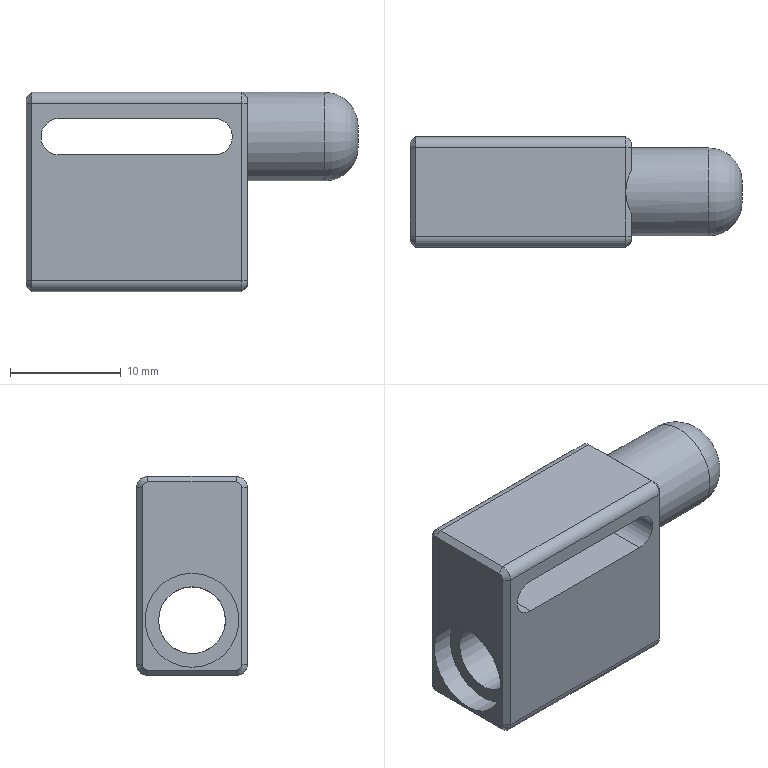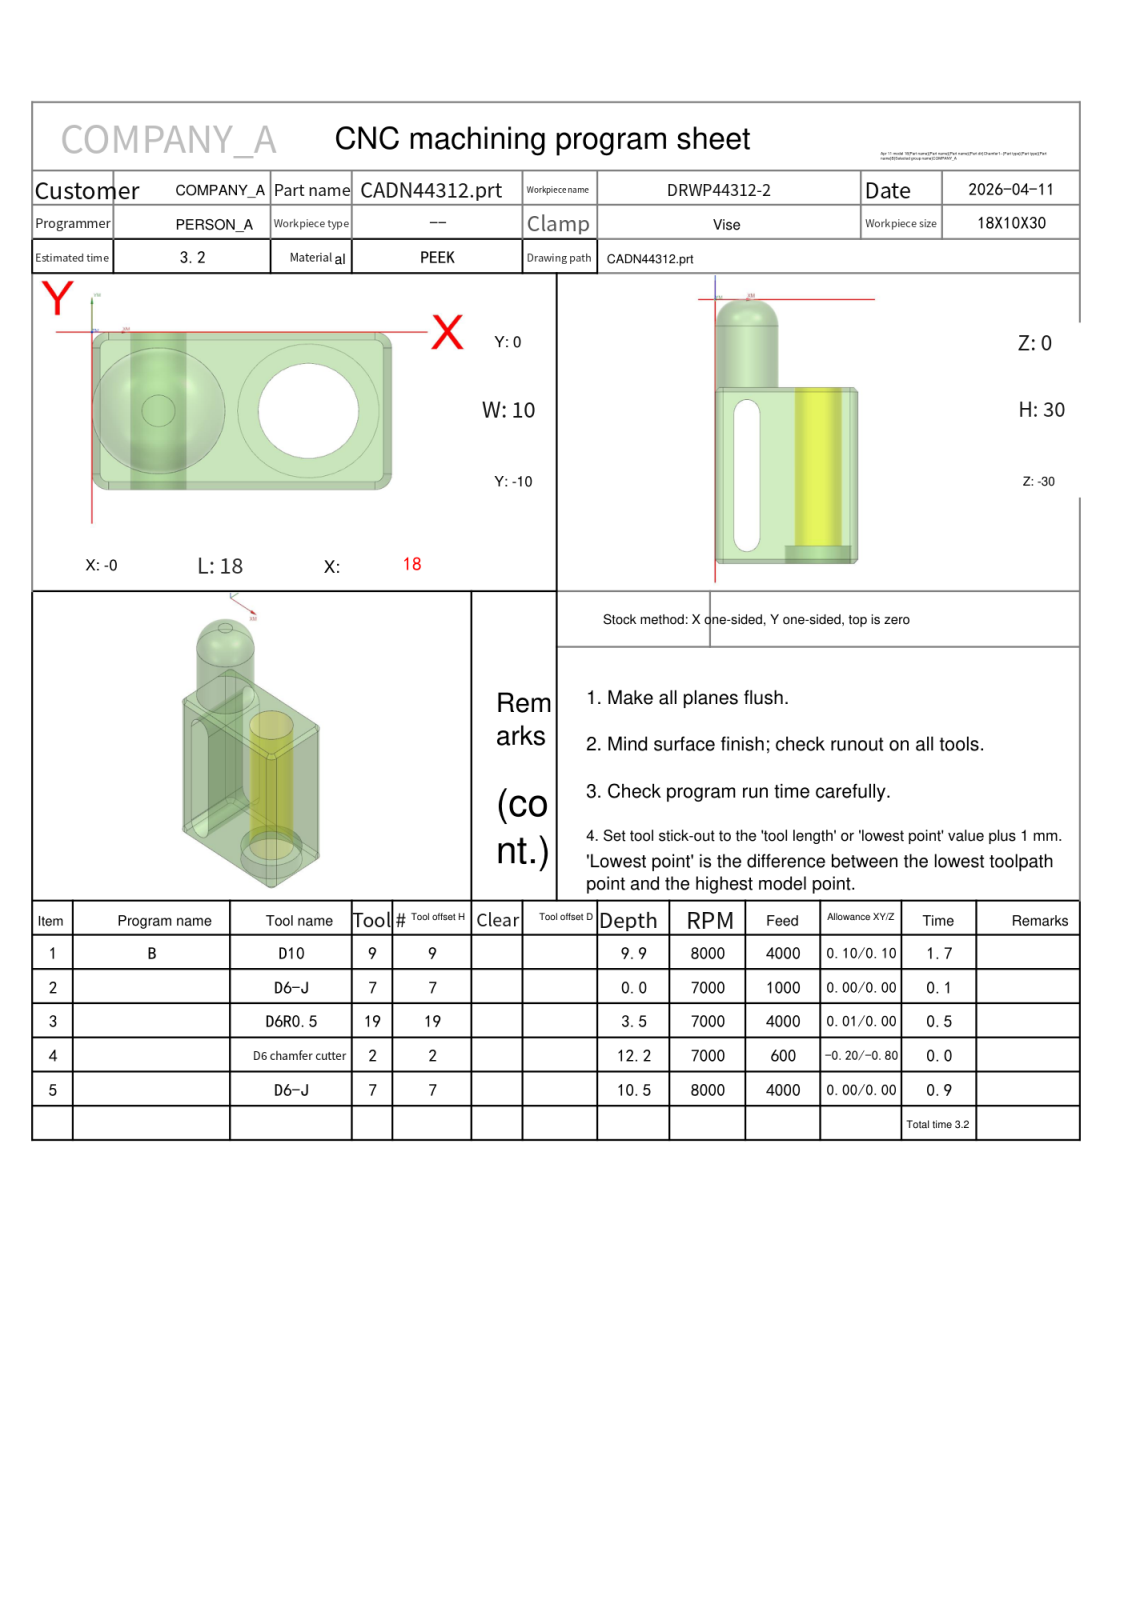NC program | NX | posted by the shop | part box 30 x 10 x 18 mm
Lines 1 to 1408 of 11854:
%
O0001
(Machine time: 4.17 MIN)
(===Total Tool:4===)
(T9=D10     D=10.  R=0.   D-  H09 Z=-9.9  )
(T7=D6-J    D=6.   R=0.   D-  H07 Z=-10.5 )
(T19=D6R0.5 D=6.   R=0.5  D-  H19 Z=-3.5  )
(T2=D6 chamfer cutter    D=6.   R=0.   D-  H02 Z=-12.2 )
G80 G90 G17 G49 G40
G91 G28 Z0
M01
N1 T09 M06
(D10  D=10. R=0. H=09 ce=0.20 di=0.10)
G00 G90 G54 X-17. Y-1.667 M03 S8000
G43 H09 Z20.
M08
Z6.011
G01 Z4.011 F3000.
X-5.
X22.
G02 X23. Y-2.666 I0.0 J-1.
G01 Y-7.433
G02 X22.1 Y-8.333 I-.9 J0.0
G01 X-5.
X-17.
Z6.011
G00 Z7.5
Y-1.667
Z5.522
G01 Z3.522
X-5.
X22.
G02 X23. Y-2.666 I0.0 J-1.
G01 Y-7.433
G02 X22.1 Y-8.333 I-.9 J0.0
G01 X-5.
X-17.
Z5.522
G00 Z7.011
Y-1.667
Z5.033
G01 Z3.033
X-5.
X22.
G02 X23. Y-2.666 I0.0 J-1.
G01 Y-7.433
G02 X22.1 Y-8.333 I-.9 J0.0
G01 X-5.
X-17.
Z5.033
G00 Z6.522
Y-1.667
Z4.544
G01 Z2.544
X-5.
X22.
G02 X23. Y-2.666 I0.0 J-1.
G01 Y-7.433
G02 X22.1 Y-8.333 I-.9 J0.0
G01 X-5.
X-17.
Z4.544
G00 Z6.033
Y-1.667
Z4.056
G01 Z2.056
X-5.
X22.
G02 X23. Y-2.666 I0.0 J-1.
G01 Y-7.433
G02 X22.1 Y-8.333 I-.9 J0.0
G01 X-5.
X-17.
Z4.056
G00 Z5.544
Y-1.667
Z3.567
G01 Z1.567
X-5.
X22.
G02 X23. Y-2.666 I0.0 J-1.
G01 Y-7.433
G02 X22.1 Y-8.333 I-.9 J0.0
G01 X-5.
X-17.
Z3.567
G00 Z5.056
Y-1.667
Z3.078
G01 Z1.078
X-5.
X22.
G02 X23. Y-2.666 I0.0 J-1.
G01 Y-7.433
G02 X22.1 Y-8.333 I-.9 J0.0
G01 X-5.
X-17.
Z3.078
G00 Z4.567
Y-1.667
Z2.589
G01 Z.589
X-5.
X22.
G02 X23. Y-2.666 I0.0 J-1.
G01 Y-7.433
G02 X22.1 Y-8.333 I-.9 J0.0
G01 X-5.
X-17.
Z2.589
G00 Z4.078
Y-1.667
Z2.1
G01 Z.1
X-5.
X22.
G02 X23. Y-2.666 I0.0 J-1.
G01 Y-7.433
G02 X22.1 Y-8.333 I-.9 J0.0
G01 X-5.
X-17.
Z2.1
G00 Z20.
G00 G90 X7.765 Y13. M03 S8000
Z14.8
Z.804
G01 Z-.396 F4000.
Y8.5
G03 X14.765 Y1.5 I7. J0.0
G01 X19.429
X20.55 Y1.496
G02 X20.998 Y1.048 I-.048 J-.495
G01 Y-11.048
G02 X20.55 Y-11.496 I-.495 J.047
G01 X19.43 Y-11.499
X10.345 Y-11.498
G02 X4. Y-14.082 I-6.345 J6.498
X-2.347 Y-11.496 I0.0 J9.082
G01 X-2.553
G02 X-2.998 Y-11.048 I.051 J.495
G01 Y-10.789
G02 X-5.082 Y-5. I6.998 J5.789
X-2.998 Y.789 I9.082 J0.0
G01 Y1.048
G02 X-2.55 Y1.496 I.495 J-.047
G01 X-2.346 Y1.497
G02 X4. Y4.082 I6.346 J-6.497
X10.343 Y1.5 I0.0 J-9.082
G01 X14.031
G02 X14.99 Y.785 I0.0 J-1.
G01 X16.144 Y-3.092
G03 X16.3 Y-3.403 I.958 J.286
G02 X16.498 Y-3.999 I-.802 J-.597
G01 Y-6.
G02 X15.499 Y-6.999 I-1. J.001
G01 X14.031
G02 X13.032 Y-5.999 I.001 J1.
G01 X13.037 Y-5.901
G03 X13.082 Y-5. I-9.037 J.901
X13.079 Y-4.775 I-9.082 J0.0
X12.449 Y-4.16 I-.63 J-.016
G01 X12.387 Y-4.163
X12.354 Y-4.167
G03 X11.682 Y-4.91 I.074 J-.743
G01 Y-4.917
Y-5.
G02 X4. Y-12.682 I-7.682 J0.0
X-3.682 Y-5. I0.0 J7.682
X4. Y2.682 I7.682 J0.0
X11.644 Y-4.238 I0.0 J-7.682
G03 X12.062 Y-4.616 I.418 J.042
X12.279 Y-4.556 I0.0 J.42
G01 X12.846 Y-4.214
G03 X13.036 Y-3.91 I-.205 J.34
G02 X14.031 Y-3. I.996 J-.091
G01 X14.531
G03 X21.531 Y3.999 I0.0 J7.
G01 Y12.955
Z.804
G00 Z3.
G01 X32.458 Y2. F6000.
G00 Z.408
G01 Z-.792 F4000.
X27.998
G03 X20.998 Y-5. I0.0 J-7.
G01 Y-11.048
G02 X20.55 Y-11.496 I-.496 J.047
G01 X19.43 Y-11.5
X11.034 Y-11.498
G02 X4. Y-14.576 I-7.034 J6.498
X-5.576 Y-5. I0.0 J9.576
X4. Y4.576 I9.576 J0.0
X11.032 Y1.5 I0.0 J-9.576
G01 X19.43
X20.55 Y1.496
G02 X20.998 Y1.048 I-.048 J-.495
G01 Y-10.
G02 X19.998 Y-11. I-1. J0.0
X19.383 Y-10.788 I0.0 J1.
G01 X15.112 Y-7.455
G03 X14.182 Y-6.937 I-2.131 J-2.732
G02 X13.529 Y-5.999 I.347 J.938
G01 X13.533 Y-5.905
G03 X13.576 Y-5. I-9.533 J.905
X13.573 Y-4.767 I-9.576 J0.0
X12.943 Y-4.153 I-.63 J-.015
G01 X12.884 Y-4.156
X12.852 Y-4.159
G03 X12.175 Y-4.903 I.071 J-.744
G01 Y-4.911
X12.176 Y-5.
G02 X4. Y-13.176 I-8.176 J0.0
X-4.176 Y-5. I0.0 J8.176
X4. Y3.176 I8.176 J0.0
X12.139 Y-4.226 I0.0 J-8.176
G03 X12.557 Y-4.607 I.418 J.04
X12.772 Y-4.547 I0.0 J.42
G01 X13.34 Y-4.209
G03 X13.533 Y-3.904 I-.205 J.343
G02 X14.527 Y-3. I.995 J-.096
G01 X15.499
G02 X16.498 Y-3.999 I-.001 J-1.
G01 Y-6.
G02 X16.307 Y-6.587 I-1. J.001
X15.926 Y-6.903 I-.809 J.588
G03 X11.919 Y-13.23 I2.994 J-6.328
X12.592 Y-16.224 I7. J0.0
G01 X15.797 Y-22.999
Z.408
G00 Z2.604
G01 X32.459 Y2. F6000.
G00 Z.012
G01 Z-1.188 F4000.
X27.998
G03 X20.998 Y-5. I0.0 J-7.
G01 Y-11.048
G02 X20.55 Y-11.497 I-.496 J.047
G01 X19.43 Y-11.5
X11.489 Y-11.498
G02 X4. Y-14.915 I-7.489 J6.498
X-5.915 Y-5. I0.0 J9.915
X4. Y4.915 I9.915 J0.0
X11.488 Y1.5 I0.0 J-9.915
G01 X19.43
X20.55 Y1.497
G02 X20.998 Y1.048 I-.048 J-.496
G01 Y-10.
G02 X19.998 Y-11. I-1. J0.0
X19.371 Y-10.779 I0.0 J1.
G01 X15.005 Y-7.267
G03 X14.423 Y-6.893 I-2.035 J-2.531
G02 X13.869 Y-5.999 I.447 J.895
G01 X13.874 Y-5.908
G03 X13.915 Y-5. I-9.874 J.908
X13.912 Y-4.763 I-9.915 J0.0
X13.283 Y-4.148 I-.63 J-.015
G01 X13.225 Y-4.151
X13.194 Y-4.153
G03 X12.515 Y-4.899 I.069 J-.745
G01 Y-4.907
Y-5.
G02 X4. Y-13.515 I-8.515 J0.0
X-4.515 Y-5. I0.0 J8.515
X4. Y3.515 I8.515 J0.0
X12.479 Y-4.219 I0.0 J-8.515
G03 X12.898 Y-4.601 I.418 J.039
X13.112 Y-4.542 I0.0 J.42
G01 X13.68 Y-4.205
G03 X13.874 Y-3.901 I-.204 J.344
G02 X14.868 Y-3. I.995 J-.099
G01 X15.499
G02 X16.498 Y-3.999 I-.001 J-1.
G01 Y-6.
G02 X16.307 Y-6.587 I-1. J.001
X15.926 Y-6.903 I-.809 J.588
G03 X11.919 Y-13.23 I2.994 J-6.328
X12.592 Y-16.224 I7. J0.0
G01 X15.797 Y-22.999
Z.012
G00 Z2.208
G01 X32.459 Y2. F6000.
G00 Z-.384
G01 Z-1.584 F4000.
X27.998
G03 X20.998 Y-5. I0.0 J-7.
G01 Y-11.048
G02 X20.55 Y-11.497 I-.496 J.047
G01 X19.43 Y-11.5
X11.807 Y-11.498
G02 X4. Y-15.158 I-7.807 J6.498
X-6.158 Y-5. I0.0 J10.158
X4. Y5.158 I10.158 J0.0
X11.806 Y1.5 I0.0 J-10.158
G01 X19.43
X20.55 Y1.497
G02 X20.998 Y1.048 I-.048 J-.496
G01 Y-10.
G02 X19.998 Y-11. I-1. J0.0
X19.359 Y-10.769 I0.0 J1.
G01 X14.97 Y-7.121
G03 X14.595 Y-6.855 I-1.976 J-2.379
G02 X14.113 Y-5.999 I.518 J.856
G01 X14.117 Y-5.91
G03 X14.158 Y-5. I-10.117 J.91
X14.155 Y-4.76 I-10.158 J0.0
X13.525 Y-4.145 I-.63 J-.015
G01 X13.469 Y-4.147
X13.439 Y-4.15
G03 X12.757 Y-4.896 I.067 J-.746
G01 Y-4.904
X12.758 Y-5.
G02 X4. Y-13.758 I-8.758 J0.0
X-4.758 Y-5. I0.0 J8.758
X4. Y3.758 I8.758 J0.0
X12.722 Y-4.214 I0.0 J-8.758
G03 X13.141 Y-4.597 I.418 J.038
X13.354 Y-4.539 I0.0 J.42
G01 X13.923 Y-4.203
G03 X14.118 Y-3.899 I-.203 J.344
G02 X15.112 Y-3. I.995 J-.101
G01 X15.499
G02 X16.498 Y-3.999 I-.001 J-1.
G01 Y-6.
G02 X16.307 Y-6.587 I-1. J.001
X15.926 Y-6.903 I-.809 J.588
G03 X11.919 Y-13.23 I2.994 J-6.328
X12.592 Y-16.224 I7. J0.0
G01 X15.797 Y-22.999
Z-.384
G00 Z1.812
G01 X32.459 Y2. F6000.
G00 Z-.78
G01 Z-1.98 F4000.
X27.998
G03 X20.998 Y-5. I0.0 J-7.
G01 Y-11.048
G02 X20.55 Y-11.497 I-.496 J.047
G01 X19.43 Y-11.5
X12.026 Y-11.499
G02 X4. Y-15.327 I-8.026 J6.498
X-6.327 Y-5. I0.0 J10.327
X4. Y5.327 I10.327 J0.0
X12.026 Y1.5 I0.0 J-10.327
G01 X19.43
X20.55 Y1.497
G02 X20.998 Y1.048 I-.048 J-.496
G01 Y-10.
G02 X19.998 Y-11. I-1. J0.0
X19.319 Y-10.734 I0.0 J1.
G01 X15.833 Y-7.508
G03 X14.913 Y-6.928 I-2.026 J-2.191
G02 X14.283 Y-5.999 I.37 J.929
G01 X14.287 Y-5.912
G03 X14.327 Y-5. I-10.287 J.912
X14.325 Y-4.758 I-10.327 J0.0
X13.695 Y-4.143 I-.63 J-.015
G01 X13.639 Y-4.145
X13.61 Y-4.148
G03 X12.927 Y-4.894 I.067 J-.747
G01 Y-4.902
Y-5.
G02 X4. Y-13.927 I-8.927 J0.0
X-4.927 Y-5. I0.0 J8.927
X4. Y3.927 I8.927 J0.0
X12.892 Y-4.211 I0.0 J-8.927
G03 X13.311 Y-4.594 I.418 J.037
X13.524 Y-4.536 I0.0 J.42
G01 X14.093 Y-4.201
G03 X14.288 Y-3.898 I-.203 J.345
G02 X15.282 Y-3. I.995 J-.103
G01 X15.499
G02 X16.498 Y-3.999 I-.001 J-1.
G01 Y-6.
G02 X16.307 Y-6.587 I-1. J.001
X15.926 Y-6.903 I-.809 J.588
G03 X11.919 Y-13.23 I2.994 J-6.328
X12.592 Y-16.224 I7. J0.0
G01 X15.797 Y-22.999
Z-.78
G00 Z1.416
G01 X32.459 Y2. F6000.
G00 Z-1.176
G01 Z-2.376 F4000.
X27.998
G03 X20.998 Y-5. I0.0 J-7.
G01 Y-11.048
G02 X20.55 Y-11.497 I-.496 J.047
G01 X19.43 Y-11.5
X12.166 Y-11.499
G02 X4. Y-15.437 I-8.166 J6.499
X-6.437 Y-5. I0.0 J10.437
X4. Y5.437 I10.437 J0.0
X12.166 Y1.5 I0.0 J-10.437
G01 X19.43
X20.55 Y1.497
G02 X20.998 Y1.048 I-.048 J-.496
G01 Y-10.
G02 X19.998 Y-11. I-1. J0.0
X19.309 Y-10.724 I0.0 J1.
G01 X15.936 Y-7.517
G03 X15.019 Y-6.926 I-2.008 J-2.112
G02 X14.393 Y-5.999 I.374 J.927
G01 X14.397 Y-5.913
G03 X14.437 Y-5. I-10.397 J.913
X14.434 Y-4.756 I-10.437 J0.0
X13.804 Y-4.141 I-.63 J-.015
G01 X13.749 Y-4.144
X13.72 Y-4.146
G03 X13.036 Y-4.893 I.066 J-.747
G01 Y-4.901
X13.037 Y-5.
G02 X4. Y-14.037 I-9.037 J0.0
X-5.037 Y-5. I0.0 J9.037
X4. Y4.037 I9.037 J0.0
X13.002 Y-4.209 I0.0 J-9.037
G03 X13.42 Y-4.592 I.418 J.037
X13.633 Y-4.535 I0.0 J.42
G01 X14.203 Y-4.2
G03 X14.398 Y-3.897 I-.203 J.345
G02 X15.392 Y-3. I.995 J-.103
G01 X15.499
G02 X16.498 Y-3.999 I-.001 J-1.
G01 Y-6.
G02 X16.307 Y-6.587 I-1. J.001
X15.926 Y-6.903 I-.809 J.588
G03 X11.919 Y-13.23 I2.994 J-6.328
X12.592 Y-16.224 I7. J0.0
G01 X15.797 Y-22.999
Z-1.176
G00 Z1.02
G01 X32.459 Y2. F6000.
G00 Z-1.572
G01 Z-2.772 F4000.
X27.998
G03 X20.998 Y-5. I0.0 J-7.
G01 Y-11.048
G02 X20.55 Y-11.497 I-.496 J.047
G01 X19.43 Y-11.5
X12.237 Y-11.499
G02 X4. Y-15.492 I-8.237 J6.499
X-6.492 Y-5. I0.0 J10.492
X4. Y5.492 I10.492 J0.0
X12.236 Y1.5 I0.0 J-10.492
G01 X19.43
X20.55 Y1.497
G02 X20.998 Y1.048 I-.048 J-.496
G01 Y-10.
G02 X19.998 Y-11. I-1. J0.0
X19.304 Y-10.719 I0.0 J1.
G01 X15.988 Y-7.521
G03 X15.072 Y-6.926 I-1.998 J-2.072
G02 X14.448 Y-5.999 I.376 J.927
G01 X14.452 Y-5.913
G03 X14.492 Y-5. I-10.452 J.913
X14.489 Y-4.756 I-10.492 J0.0
X13.859 Y-4.14 I-.63 J-.015
G01 X13.804 Y-4.143
X13.775 Y-4.145
G03 X13.091 Y-4.892 I.066 J-.747
G01 Y-4.9
X13.092 Y-5.
G02 X4. Y-14.092 I-9.092 J0.0
X-5.092 Y-5. I0.0 J9.092
X4. Y4.092 I9.092 J0.0
X13.057 Y-4.208 I0.0 J-9.092
G03 X13.475 Y-4.592 I.418 J.037
X13.688 Y-4.534 I0.0 J.42
G01 X14.258 Y-4.2
G03 X14.453 Y-3.896 I-.202 J.345
G02 X15.447 Y-3. I.995 J-.104
G01 X15.499
G02 X16.498 Y-3.999 I-.001 J-1.
G01 Y-6.
G02 X16.307 Y-6.587 I-1. J.001
X15.926 Y-6.903 I-.809 J.588
G03 X11.92 Y-13.231 I2.994 J-6.328
X12.592 Y-16.224 I7. J0.0
G01 X15.797 Y-22.999
Z-1.572
G00 Z.624
G01 X32.459 Y2. F6000.
G00 Z-1.968
G01 Z-3.168 F4000.
X27.998
G03 X20.998 Y-5. I0.0 J-7.
G01 Y-11.048
G02 X20.55 Y-11.497 I-.496 J.047
G01 X19.43 Y-11.5
X12.247 Y-11.499
G02 X4. Y-15.5 I-8.247 J6.499
X-6.5 Y-5. I0.0 J10.5
X4. Y5.5 I10.5 J0.0
X12.246 Y1.5 I0.0 J-10.5
G01 X19.43
X20.55 Y1.497
G02 X20.998 Y1.048 I-.048 J-.496
G01 Y-10.
G02 X19.998 Y-11. I-1. J0.0
X19.303 Y-10.719 I0.0 J1.
G01 X15.996 Y-7.522
G03 X15.08 Y-6.926 I-1.997 J-2.066
G02 X14.457 Y-5.999 I.376 J.927
G01 X14.46 Y-5.913
G03 X14.5 Y-5. I-10.46 J.913
X14.497 Y-4.756 I-10.5 J0.0
X13.867 Y-4.14 I-.63 J-.015
G01 X13.812 Y-4.143
X13.784 Y-4.145
G03 X13.099 Y-4.892 I.066 J-.747
G01 Y-4.9
X13.1 Y-5.
G02 X4. Y-14.1 I-9.1 J0.0
X-5.1 Y-5. I0.0 J9.1
X4. Y4.1 I9.1 J0.0
X13.065 Y-4.208 I0.0 J-9.1
G03 X13.484 Y-4.591 I.418 J.037
X13.696 Y-4.534 I0.0 J.42
G01 X14.266 Y-4.2
G03 X14.462 Y-3.896 I-.202 J.345
G02 X15.455 Y-3. I.995 J-.104
G01 X15.499
G02 X16.498 Y-3.999 I-.001 J-1.
G01 Y-6.
G02 X16.307 Y-6.587 I-1. J.001
X15.926 Y-6.903 I-.809 J.588
G03 X11.92 Y-13.231 I2.994 J-6.328
X12.592 Y-16.224 I7. J0.0
G01 X15.797 Y-22.999
Z-1.968
G00 Z.228
G01 X32.459 Y2. F6000.
G00 Z-2.364
G01 Z-3.564 F4000.
X27.998
G03 X20.998 Y-5. I0.0 J-7.
G01 Y-11.048
G02 X20.55 Y-11.497 I-.496 J.047
G01 X19.43 Y-11.5
X12.247 Y-11.499
G02 X4. Y-15.5 I-8.247 J6.499
X-6.5 Y-5. I0.0 J10.5
X4. Y5.5 I10.5 J0.0
X12.246 Y1.5 I0.0 J-10.5
G01 X19.43
X20.55 Y1.497
G02 X20.998 Y1.048 I-.048 J-.496
G01 Y-10.
G02 X19.998 Y-11. I-1. J0.0
X19.303 Y-10.719 I0.0 J1.
G01 X15.996 Y-7.522
G03 X15.08 Y-6.926 I-1.997 J-2.066
G02 X14.457 Y-5.999 I.376 J.927
G01 X14.46 Y-5.913
G03 X14.5 Y-5. I-10.46 J.913
X14.497 Y-4.756 I-10.5 J0.0
X13.867 Y-4.14 I-.63 J-.015
G01 X13.812 Y-4.143
X13.784 Y-4.145
G03 X13.099 Y-4.892 I.066 J-.747
G01 Y-4.9
X13.1 Y-5.
G02 X4. Y-14.1 I-9.1 J0.0
X-5.1 Y-5. I0.0 J9.1
X4. Y4.1 I9.1 J0.0
X13.065 Y-4.208 I0.0 J-9.1
G03 X13.484 Y-4.591 I.418 J.037
X13.696 Y-4.534 I0.0 J.42
G01 X14.266 Y-4.2
G03 X14.462 Y-3.896 I-.202 J.345
G02 X15.455 Y-3. I.995 J-.104
G01 X15.499
G02 X16.498 Y-3.999 I-.001 J-1.
G01 Y-6.
G02 X16.307 Y-6.587 I-1. J.001
X15.926 Y-6.903 I-.809 J.588
G03 X11.92 Y-13.231 I2.994 J-6.327
X12.592 Y-16.224 I7. J0.0
G01 X15.798 Y-22.999
Z-2.364
G00 Z-.168
G01 X32.459 Y2. F6000.
G00 Z-2.76
G01 Z-3.96 F4000.
X27.998
G03 X20.998 Y-5. I0.0 J-7.
G01 Y-11.048
G02 X20.55 Y-11.497 I-.496 J.047
G01 X19.43 Y-11.5
X12.247 Y-11.499
G02 X4. Y-15.5 I-8.247 J6.499
X-6.5 Y-5. I0.0 J10.5
X4. Y5.5 I10.5 J0.0
X12.246 Y1.5 I0.0 J-10.5
G01 X19.43
X20.55 Y1.497
G02 X20.998 Y1.048 I-.048 J-.496
G01 Y-10.
G02 X19.998 Y-11. I-1. J0.0
X19.303 Y-10.719 I0.0 J1.
G01 X15.996 Y-7.522
G03 X15.08 Y-6.926 I-1.997 J-2.067
G02 X14.457 Y-5.999 I.376 J.927
G01 X14.46 Y-5.913
G03 X14.5 Y-5. I-10.46 J.913
X14.497 Y-4.756 I-10.5 J0.0
X13.867 Y-4.14 I-.63 J-.015
G01 X13.812 Y-4.143
X13.784 Y-4.145
G03 X13.099 Y-4.892 I.066 J-.747
G01 Y-4.9
X13.1 Y-5.
G02 X4. Y-14.1 I-9.1 J0.0
X-5.1 Y-5. I0.0 J9.1
X4. Y4.1 I9.1 J0.0
X13.065 Y-4.208 I0.0 J-9.1
G03 X13.484 Y-4.591 I.418 J.037
X13.696 Y-4.534 I0.0 J.42
G01 X14.266 Y-4.2
G03 X14.462 Y-3.896 I-.202 J.345
G02 X15.455 Y-3. I.995 J-.104
G01 X15.499
G02 X16.498 Y-3.999 I-.001 J-1.
G01 Y-6.
G02 X16.307 Y-6.587 I-1. J.001
X15.926 Y-6.903 I-.809 J.588
G03 X11.92 Y-13.231 I2.994 J-6.327
X12.592 Y-16.224 I7. J0.0
G01 X15.798 Y-22.999
Z-2.76
G00 Z-.564
G01 X32.459 Y2. F6000.
G00 Z-3.156
G01 Z-4.356 F4000.
X27.998
G03 X20.998 Y-5. I0.0 J-7.
G01 Y-11.048
G02 X20.55 Y-11.497 I-.496 J.047
G01 X19.43 Y-11.5
X12.247 Y-11.499
G02 X4. Y-15.5 I-8.247 J6.499
X-6.5 Y-5. I0.0 J10.5
X4. Y5.5 I10.5 J0.0
X12.246 Y1.5 I0.0 J-10.5
G01 X19.43
X20.55 Y1.497
G02 X20.998 Y1.048 I-.048 J-.496
G01 Y-10.
G02 X19.998 Y-11. I-1. J0.0
X19.303 Y-10.719 I0.0 J1.
G01 X15.996 Y-7.522
G03 X15.08 Y-6.926 I-1.997 J-2.067
G02 X14.457 Y-5.999 I.376 J.927
G01 X14.46 Y-5.913
G03 X14.5 Y-5. I-10.46 J.913
X14.497 Y-4.756 I-10.5 J0.0
X13.867 Y-4.14 I-.63 J-.015
G01 X13.812 Y-4.143
X13.784 Y-4.145
G03 X13.099 Y-4.892 I.066 J-.747
G01 Y-4.9
X13.1 Y-5.
G02 X4. Y-14.1 I-9.1 J0.0
X-5.1 Y-5. I0.0 J9.1
X4. Y4.1 I9.1 J0.0
X13.065 Y-4.208 I0.0 J-9.1
G03 X13.484 Y-4.591 I.418 J.037
X13.696 Y-4.534 I0.0 J.42
G01 X14.266 Y-4.2
G03 X14.462 Y-3.896 I-.202 J.345
G02 X15.455 Y-3. I.995 J-.104
G01 X15.499
G02 X16.498 Y-3.999 I-.001 J-1.
G01 Y-6.
G02 X16.307 Y-6.587 I-1. J.001
X15.926 Y-6.903 I-.809 J.588
G03 X11.92 Y-13.231 I2.994 J-6.327
X12.592 Y-16.224 I7. J0.0
G01 X15.798 Y-22.999
Z-3.156
G00 Z-.96
G01 X32.459 Y2. F6000.
G00 Z-3.552
G01 Z-4.752 F4000.
X27.998
G03 X20.998 Y-5. I0.0 J-7.
G01 Y-11.048
G02 X20.55 Y-11.497 I-.496 J.047
G01 X19.43 Y-11.5
X12.247 Y-11.499
G02 X4. Y-15.5 I-8.247 J6.499
X-6.5 Y-5. I0.0 J10.5
X4. Y5.5 I10.5 J0.0
X12.246 Y1.5 I0.0 J-10.5
G01 X19.43
X20.55 Y1.497
G02 X20.998 Y1.048 I-.048 J-.496
G01 Y-10.
G02 X19.998 Y-11. I-1. J0.0
X19.303 Y-10.719 I0.0 J1.
G01 X15.996 Y-7.522
G03 X15.08 Y-6.926 I-1.997 J-2.067
G02 X14.457 Y-5.999 I.376 J.927
G01 X14.46 Y-5.913
G03 X14.5 Y-5. I-10.46 J.913
X14.497 Y-4.756 I-10.5 J0.0
X13.867 Y-4.14 I-.63 J-.015
G01 X13.812 Y-4.143
X13.784 Y-4.145
G03 X13.099 Y-4.892 I.066 J-.747
G01 Y-4.9
X13.1 Y-5.
G02 X4. Y-14.1 I-9.1 J0.0
X-5.1 Y-5. I0.0 J9.1
X4. Y4.1 I9.1 J0.0
X13.065 Y-4.208 I0.0 J-9.1
G03 X13.484 Y-4.591 I.418 J.037
X13.696 Y-4.534 I0.0 J.42
G01 X14.266 Y-4.2
G03 X14.462 Y-3.896 I-.202 J.345
G02 X15.455 Y-3. I.995 J-.104
G01 X15.499
G02 X16.498 Y-3.999 I-.001 J-1.
G01 Y-6.
G02 X16.307 Y-6.587 I-1. J.001
X15.926 Y-6.903 I-.809 J.588
G03 X11.92 Y-13.231 I2.994 J-6.327
X12.592 Y-16.224 I7. J0.0
G01 X15.798 Y-22.999
Z-3.552
G00 Z-1.356
G01 X32.459 Y2. F6000.
G00 Z-3.948
G01 Z-5.148 F4000.
X27.998
G03 X20.998 Y-5. I0.0 J-7.
G01 Y-11.048
G02 X20.55 Y-11.497 I-.497 J.047
G01 X19.431 Y-11.5
X12.247 Y-11.499
G02 X4. Y-15.5 I-8.247 J6.499
X-6.5 Y-5. I0.0 J10.5
X4. Y5.5 I10.5 J0.0
X12.246 Y1.5 I0.0 J-10.5
G01 X19.43
X20.55 Y1.497
G02 X20.998 Y1.048 I-.048 J-.496
G01 Y-10.
G02 X19.998 Y-11. I-1. J0.0
X19.303 Y-10.719 I0.0 J1.
G01 X15.996 Y-7.522
G03 X15.08 Y-6.926 I-1.997 J-2.067
G02 X14.457 Y-5.999 I.376 J.927
G01 X14.46 Y-5.913
G03 X14.5 Y-5. I-10.46 J.913
X14.497 Y-4.756 I-10.5 J0.0
X13.867 Y-4.14 I-.63 J-.015
G01 X13.812 Y-4.143
X13.784 Y-4.145
G03 X13.099 Y-4.892 I.066 J-.747
G01 Y-4.9
X13.1 Y-5.
G02 X4. Y-14.1 I-9.1 J0.0
X-5.1 Y-5. I0.0 J9.1
X4. Y4.1 I9.1 J0.0
X13.065 Y-4.208 I0.0 J-9.1
G03 X13.484 Y-4.591 I.418 J.037
X13.696 Y-4.534 I0.0 J.42
G01 X14.266 Y-4.2
G03 X14.462 Y-3.896 I-.202 J.345
G02 X15.455 Y-3. I.995 J-.104
G01 X15.499
G02 X16.498 Y-3.999 I-.001 J-1.
G01 Y-6.
G02 X16.307 Y-6.587 I-1. J.001
X15.926 Y-6.903 I-.809 J.588
G03 X11.92 Y-13.231 I2.994 J-6.327
X12.592 Y-16.224 I7. J0.0
G01 X15.798 Y-22.999
Z-3.948
G00 Z-1.752
G01 X32.459 Y2. F6000.
G00 Z-4.344
G01 Z-5.544 F4000.
X27.998
G03 X20.998 Y-5. I0.0 J-7.
G01 Y-11.048
G02 X20.55 Y-11.497 I-.497 J.047
G01 X19.431 Y-11.5
X12.247 Y-11.499
G02 X4. Y-15.5 I-8.247 J6.499
X-6.5 Y-5. I0.0 J10.5
X4. Y5.5 I10.5 J0.0
X12.246 Y1.5 I0.0 J-10.5
G01 X19.43
X20.55 Y1.497
G02 X20.998 Y1.048 I-.048 J-.496
G01 Y-10.
G02 X19.998 Y-11. I-1. J0.0
X19.303 Y-10.719 I0.0 J1.
G01 X15.996 Y-7.522
G03 X15.08 Y-6.926 I-1.997 J-2.067
G02 X14.457 Y-5.999 I.376 J.927
G01 X14.46 Y-5.913
G03 X14.5 Y-5. I-10.46 J.913
X14.497 Y-4.756 I-10.5 J0.0
X13.867 Y-4.14 I-.63 J-.015
G01 X13.812 Y-4.143
X13.784 Y-4.145
G03 X13.099 Y-4.892 I.066 J-.747
G01 Y-4.9
X13.1 Y-5.
G02 X4. Y-14.1 I-9.1 J0.0
X-5.1 Y-5. I0.0 J9.1
X4. Y4.1 I9.1 J0.0
X13.065 Y-4.208 I0.0 J-9.1
G03 X13.484 Y-4.591 I.418 J.037
X13.696 Y-4.534 I0.0 J.42
G01 X14.266 Y-4.2
G03 X14.462 Y-3.896 I-.202 J.345
G02 X15.455 Y-3. I.995 J-.104
G01 X15.499
G02 X16.498 Y-3.999 I-.001 J-1.
G01 Y-6.
G02 X16.307 Y-6.587 I-1. J.001
X15.926 Y-6.903 I-.809 J.588
G03 X11.92 Y-13.231 I2.994 J-6.327
X12.592 Y-16.225 I7. J0.0
G01 X15.798 Y-22.999
Z-4.344
G00 Z-2.148
G01 X32.459 Y2. F6000.
G00 Z-4.74
G01 Z-5.94 F4000.
X27.998
G03 X20.998 Y-5. I0.0 J-7.
G01 Y-11.048
G02 X20.55 Y-11.497 I-.497 J.047
G01 X19.431 Y-11.5
X12.247 Y-11.499
G02 X4. Y-15.5 I-8.247 J6.499
X-6.5 Y-5. I0.0 J10.5
X4. Y5.5 I10.5 J0.0
X12.246 Y1.5 I0.0 J-10.5
G01 X19.43
X20.55 Y1.497
G02 X20.998 Y1.048 I-.049 J-.497
G01 Y-10.
G02 X19.998 Y-11. I-1. J0.0
X19.303 Y-10.719 I0.0 J1.
G01 X15.996 Y-7.522
G03 X15.08 Y-6.926 I-1.997 J-2.067
G02 X14.457 Y-5.999 I.376 J.927
G01 X14.46 Y-5.914
G03 X14.5 Y-5. I-10.46 J.914
X14.497 Y-4.756 I-10.5 J0.0
X13.867 Y-4.14 I-.63 J-.015
G01 X13.812 Y-4.143
X13.784 Y-4.145
G03 X13.099 Y-4.892 I.066 J-.747
G01 Y-4.9
X13.1 Y-5.
G02 X4. Y-14.1 I-9.1 J0.0
X-5.1 Y-5. I0.0 J9.1
X4. Y4.1 I9.1 J0.0
X13.065 Y-4.208 I0.0 J-9.1
G03 X13.484 Y-4.591 I.418 J.037
X13.696 Y-4.534 I0.0 J.42
G01 X14.266 Y-4.2
G03 X14.462 Y-3.896 I-.202 J.345
G02 X15.455 Y-3. I.995 J-.104
G01 X15.499
G02 X16.498 Y-3.999 I-.001 J-1.
G01 Y-6.
G02 X16.307 Y-6.588 I-1. J.001
X15.926 Y-6.903 I-.809 J.588
G03 X11.92 Y-13.231 I2.994 J-6.327
X12.592 Y-16.225 I7. J0.0
G01 X15.798 Y-22.999
Z-4.74
G00 Z-2.544
G01 X32.459 Y2. F6000.
G00 Z-5.136
G01 Z-6.336 F4000.
X27.998
G03 X20.998 Y-5. I0.0 J-7.
G01 Y-11.048
G02 X20.55 Y-11.497 I-.497 J.047
G01 X19.431 Y-11.5
X12.247 Y-11.499
G02 X4. Y-15.5 I-8.247 J6.499
X-6.5 Y-5. I0.0 J10.5
X4. Y5.5 I10.5 J0.0
X12.246 Y1.5 I0.0 J-10.5
G01 X19.43
X20.55 Y1.497
G02 X20.998 Y1.048 I-.049 J-.497
G01 Y-10.
G02 X19.998 Y-11. I-1. J0.0
X19.303 Y-10.719 I0.0 J1.
G01 X15.996 Y-7.522
G03 X15.08 Y-6.926 I-1.997 J-2.067
G02 X14.456 Y-5.999 I.376 J.927
G01 X14.46 Y-5.914
G03 X14.5 Y-5. I-10.46 J.914
X14.497 Y-4.756 I-10.5 J0.0
X13.867 Y-4.14 I-.63 J-.015
G01 X13.812 Y-4.143
X13.784 Y-4.145
G03 X13.099 Y-4.892 I.066 J-.747
G01 Y-4.9
X13.1 Y-5.
G02 X4. Y-14.1 I-9.1 J0.0
X-5.1 Y-5. I0.0 J9.1
X4. Y4.1 I9.1 J0.0
X13.065 Y-4.208 I0.0 J-9.1
G03 X13.484 Y-4.591 I.418 J.037
X13.696 Y-4.534 I0.0 J.42
G01 X14.266 Y-4.2
G03 X14.462 Y-3.896 I-.202 J.345
G02 X15.455 Y-3. I.995 J-.104
G01 X15.499
G02 X16.498 Y-3.999 I-.001 J-1.
G01 Y-6.
G02 X16.307 Y-6.588 I-1. J.001
X15.926 Y-6.903 I-.809 J.588
G03 X11.92 Y-13.231 I2.994 J-6.327
X12.592 Y-16.225 I7. J0.0
G01 X15.798 Y-22.999
Z-5.136
G00 Z-2.94
G01 X32.459 Y2. F6000.
G00 Z-5.532
G01 Z-6.732 F4000.
X27.998
G03 X20.998 Y-5. I0.0 J-7.
G01 Y-11.048
G02 X20.55 Y-11.497 I-.497 J.047
G01 X19.431 Y-11.5
X12.247 Y-11.499
G02 X4. Y-15.5 I-8.247 J6.499
X-6.5 Y-5. I0.0 J10.5
X4. Y5.5 I10.5 J0.0
X12.246 Y1.5 I0.0 J-10.5
G01 X19.43
X20.55 Y1.497
G02 X20.998 Y1.048 I-.049 J-.497
G01 Y-10.
G02 X19.998 Y-11. I-1. J0.0
X19.303 Y-10.719 I0.0 J1.
G01 X15.996 Y-7.522
G03 X15.08 Y-6.926 I-1.997 J-2.067
G02 X14.456 Y-5.999 I.376 J.927
G01 X14.46 Y-5.914
G03 X14.5 Y-5. I-10.46 J.914
X14.497 Y-4.756 I-10.5 J0.0
X13.867 Y-4.14 I-.63 J-.015
G01 X13.812 Y-4.143
X13.784 Y-4.145
G03 X13.099 Y-4.892 I.066 J-.747
G01 Y-4.9
X13.1 Y-5.
G02 X4. Y-14.1 I-9.1 J0.0
X-5.1 Y-5. I0.0 J9.1
X4. Y4.1 I9.1 J0.0
X13.065 Y-4.208 I0.0 J-9.1
G03 X13.484 Y-4.591 I.418 J.037
X13.696 Y-4.534 I0.0 J.42
G01 X14.266 Y-4.199
G03 X14.462 Y-3.896 I-.202 J.345
G02 X15.455 Y-3. I.995 J-.104
G01 X15.499
G02 X16.498 Y-3.999 I-.001 J-1.
G01 Y-6.001
G02 X16.307 Y-6.588 I-1. J.001
X15.926 Y-6.903 I-.809 J.588
G03 X11.92 Y-13.231 I2.994 J-6.327
X12.593 Y-16.225 I7. J0.0
G01 X15.798 Y-22.999
Z-5.532
G00 Z-3.336
G01 X32.459 Y2. F6000.
G00 Z-5.928
G01 Z-7.128 F4000.
X27.998
G03 X20.998 Y-5. I0.0 J-7.
G01 Y-11.048
G02 X20.55 Y-11.497 I-.497 J.047
G01 X19.431 Y-11.5
X12.247 Y-11.499
G02 X4. Y-15.5 I-8.247 J6.499
X-6.5 Y-5. I0.0 J10.5
X4. Y5.5 I10.5 J0.0
X12.246 Y1.5 I0.0 J-10.5
G01 X19.431
X20.55 Y1.497
G02 X20.998 Y1.048 I-.049 J-.497
G01 Y-10.
G02 X19.998 Y-11. I-1. J0.0
X19.303 Y-10.719 I0.0 J1.
G01 X15.996 Y-7.522
G03 X15.08 Y-6.926 I-1.997 J-2.067
G02 X14.456 Y-5.999 I.376 J.927
G01 X14.46 Y-5.914
G03 X14.5 Y-5. I-10.46 J.914
X14.497 Y-4.755 I-10.5 J0.0
X13.867 Y-4.14 I-.63 J-.015
G01 X13.812 Y-4.143
X13.784 Y-4.145
G03 X13.099 Y-4.892 I.066 J-.747
G01 Y-4.9
X13.1 Y-5.
G02 X4. Y-14.1 I-9.1 J0.0
X-5.1 Y-5. I0.0 J9.1
X4. Y4.1 I9.1 J0.0
X13.065 Y-4.208 I0.0 J-9.1
G03 X13.484 Y-4.591 I.418 J.037
X13.696 Y-4.534 I0.0 J.42
G01 X14.266 Y-4.199
G03 X14.462 Y-3.896 I-.202 J.345
G02 X15.455 Y-3. I.995 J-.104
G01 X15.499
G02 X16.498 Y-3.999 I-.001 J-1.
G01 Y-6.001
G02 X16.307 Y-6.588 I-1. J.001
X15.926 Y-6.903 I-.809 J.588
G03 X11.92 Y-13.231 I2.994 J-6.327
X12.593 Y-16.225 I7. J0.0
G01 X15.798 Y-22.999
Z-5.928
G00 Z-3.732
G01 X32.459 Y2. F6000.
G00 Z-6.324
G01 Z-7.524 F4000.
X27.998
G03 X20.998 Y-5. I0.0 J-7.
G01 Y-11.048
G02 X20.55 Y-11.497 I-.497 J.047
G01 X19.431 Y-11.5
X12.247 Y-11.499
G02 X4. Y-15.5 I-8.247 J6.499
X-6.5 Y-5. I0.0 J10.5
X4. Y5.5 I10.5 J0.0
X12.246 Y1.5 I0.0 J-10.5
G01 X19.431
X20.55 Y1.497
G02 X20.998 Y1.048 I-.049 J-.497
G01 Y-10.
G02 X19.998 Y-11. I-1. J0.0
X19.303 Y-10.719 I0.0 J1.
G01 X15.996 Y-7.522
G03 X15.08 Y-6.926 I-1.997 J-2.067
G02 X14.456 Y-5.999 I.376 J.927
G01 X14.46 Y-5.914
G03 X14.5 Y-5. I-10.46 J.914
X14.497 Y-4.755 I-10.5 J0.0
X13.867 Y-4.14 I-.63 J-.015
G01 X13.812 Y-4.143
X13.784 Y-4.145
G03 X13.099 Y-4.892 I.066 J-.747
G01 Y-4.9
X13.1 Y-5.
G02 X4. Y-14.1 I-9.1 J0.0
X-5.1 Y-5. I0.0 J9.1
X4. Y4.1 I9.1 J0.0
X13.065 Y-4.208 I0.0 J-9.1
G03 X13.484 Y-4.591 I.418 J.037
X13.696 Y-4.534 I0.0 J.42
G01 X14.266 Y-4.199
G03 X14.462 Y-3.896 I-.202 J.345
G02 X15.455 Y-3. I.995 J-.104
G01 X15.5
G02 X16.498 Y-3.999 I-.001 J-1.
G01 Y-6.001
G02 X16.307 Y-6.588 I-1. J.001
X15.926 Y-6.903 I-.809 J.588
G03 X11.92 Y-13.231 I2.994 J-6.327
X12.593 Y-16.225 I7. J0.0
G01 X15.798 Y-22.999
Z-6.324
G00 Z-4.128
G01 X32.459 Y2. F6000.
G00 Z-6.72
G01 Z-7.92 F4000.
X27.998
G03 X20.998 Y-5. I0.0 J-7.
G01 Y-11.048
G02 X20.55 Y-11.497 I-.497 J.047
G01 X19.431 Y-11.5
X12.247 Y-11.499
G02 X4. Y-15.5 I-8.247 J6.499
X-6.5 Y-5. I0.0 J10.5
X4. Y5.5 I10.5 J0.0
X12.246 Y1.5 I0.0 J-10.5
G01 X19.431
X20.55 Y1.497
G02 X20.998 Y1.048 I-.049 J-.497
G01 Y-10.
G02 X19.998 Y-11. I-1. J0.0
X19.303 Y-10.719 I0.0 J1.
G01 X15.996 Y-7.522
G03 X15.08 Y-6.926 I-1.997 J-2.067
G02 X14.456 Y-5.999 I.376 J.927
G01 X14.46 Y-5.914
G03 X14.5 Y-5. I-10.46 J.914
X14.497 Y-4.755 I-10.5 J0.0
X13.867 Y-4.14 I-.63 J-.015
G01 X13.812 Y-4.143
X13.784 Y-4.145
G03 X13.099 Y-4.892 I.066 J-.747
G01 Y-4.9
X13.1 Y-5.
G02 X4. Y-14.1 I-9.1 J0.0
X-5.1 Y-5. I0.0 J9.1
X4. Y4.1 I9.1 J0.0
X13.065 Y-4.208 I0.0 J-9.1
G03 X13.484 Y-4.591 I.418 J.037
X13.696 Y-4.534 I0.0 J.42
G01 X14.266 Y-4.199
G03 X14.462 Y-3.896 I-.202 J.345
G02 X15.455 Y-3. I.995 J-.104
G01 X15.5
G02 X16.498 Y-3.999 I-.001 J-1.
G01 Y-6.001
G02 X16.307 Y-6.588 I-1. J.001
X15.926 Y-6.903 I-.809 J.588
G03 X11.92 Y-13.231 I2.994 J-6.327
X12.593 Y-16.225 I7. J0.0
G01 X15.798 Y-22.999
Z-6.72
G00 Z-4.524
G01 X32.459 Y2. F6000.
G00 Z-7.116
G01 Z-8.316 F4000.
X27.998
G03 X20.998 Y-5. I0.0 J-7.
G01 Y-11.048
G02 X20.55 Y-11.497 I-.497 J.047
G01 X19.431 Y-11.5
X12.247 Y-11.499
G02 X4. Y-15.5 I-8.247 J6.499
X-6.5 Y-5. I0.0 J10.5
X4. Y5.5 I10.5 J0.0
X12.246 Y1.5 I0.0 J-10.5
G01 X19.431
X20.55 Y1.497
G02 X20.998 Y1.048 I-.049 J-.497
G01 Y-10.
G02 X19.998 Y-11. I-1. J0.0
X19.303 Y-10.719 I0.0 J1.
G01 X15.996 Y-7.522
G03 X15.08 Y-6.926 I-1.997 J-2.067
G02 X14.456 Y-5.999 I.376 J.927
G01 X14.46 Y-5.914
G03 X14.5 Y-5. I-10.46 J.914
X14.497 Y-4.755 I-10.5 J0.0
X13.867 Y-4.14 I-.63 J-.015
G01 X13.812 Y-4.142
X13.784 Y-4.145
G03 X13.099 Y-4.892 I.066 J-.747
G01 Y-4.9
X13.1 Y-5.
G02 X4. Y-14.1 I-9.1 J0.0
X-5.1 Y-5. I0.0 J9.1
X4. Y4.1 I9.1 J0.0
X13.065 Y-4.208 I0.0 J-9.1
G03 X13.484 Y-4.591 I.418 J.037
X13.696 Y-4.534 I0.0 J.42
G01 X14.266 Y-4.199
G03 X14.462 Y-3.896 I-.202 J.345
G02 X15.455 Y-3. I.995 J-.104
G01 X15.5
G02 X16.498 Y-3.999 I-.001 J-1.
G01 Y-6.001
G02 X16.307 Y-6.588 I-1. J.001
X15.926 Y-6.903 I-.809 J.588
G03 X11.92 Y-13.231 I2.994 J-6.327
X12.593 Y-16.225 I7. J0.0
G01 X15.798 Y-23.
Z-7.116
G00 Z-4.92
G01 X32.459 Y2. F6000.
G00 Z-7.512
G01 Z-8.712 F4000.
X27.998
G03 X20.998 Y-5. I0.0 J-7.
G01 Y-11.048
G02 X20.55 Y-11.498 I-.497 J.047
G01 X19.431 Y-11.5
X12.247 Y-11.499
G02 X4. Y-15.5 I-8.247 J6.499
X-6.5 Y-5. I0.0 J10.5
X4. Y5.5 I10.5 J0.0
X12.246 Y1.5 I0.0 J-10.5
G01 X19.431
X20.55 Y1.498
G02 X20.998 Y1.048 I-.049 J-.497
G01 Y-10.
G02 X19.998 Y-11. I-1. J0.0
X19.303 Y-10.719 I0.0 J1.
G01 X15.996 Y-7.522
G03 X15.08 Y-6.926 I-1.997 J-2.067
G02 X14.456 Y-5.999 I.376 J.927
G01 X14.46 Y-5.914
G03 X14.5 Y-5. I-10.46 J.914
X14.497 Y-4.755 I-10.5 J0.0
X13.867 Y-4.14 I-.63 J-.015
G01 X13.812 Y-4.142
X13.784 Y-4.145
G03 X13.099 Y-4.892 I.066 J-.747
G01 Y-4.9
X13.1 Y-5.
G02 X4. Y-14.1 I-9.1 J0.0
X-5.1 Y-5. I0.0 J9.1
X4. Y4.1 I9.1 J0.0
X13.065 Y-4.208 I0.0 J-9.1
G03 X13.484 Y-4.591 I.418 J.037
X13.696 Y-4.534 I0.0 J.42
G01 X14.266 Y-4.199
G03 X14.462 Y-3.896 I-.202 J.345
G02 X15.455 Y-3. I.995 J-.104
G01 X15.5
G02 X16.498 Y-3.999 I-.001 J-1.
G01 Y-6.001
G02 X16.307 Y-6.588 I-1. J.001
X15.926 Y-6.903 I-.809 J.588
G03 X11.92 Y-13.231 I2.994 J-6.327
X12.593 Y-16.225 I7. J0.0
G01 X15.799 Y-23.
Z-7.512
G00 Z-5.316
G01 X32.459 Y2. F6000.
G00 Z-7.908
G01 Z-9.108 F4000.
X27.998
G03 X20.998 Y-5. I0.0 J-7.
G01 Y-11.048
G02 X20.55 Y-11.498 I-.497 J.047
G01 X19.431 Y-11.5
X12.246
G02 X4. Y-15.5 I-8.246 J6.5
X-6.5 Y-5. I0.0 J10.5
X4. Y5.5 I10.5 J0.0
X12.246 Y1.5 I0.0 J-10.5
G01 X19.431
X20.55 Y1.498
G02 X20.998 Y1.048 I-.049 J-.497
G01 Y-10.
G02 X19.998 Y-11. I-1. J0.0
X19.303 Y-10.719 I0.0 J1.
G01 X15.996 Y-7.523
G03 X15.08 Y-6.927 I-1.997 J-2.067
G02 X14.456 Y-6. I.376 J.927
G01 X14.46 Y-5.914
G03 X14.5 Y-5. I-10.46 J.914
X14.497 Y-4.755 I-10.5 J0.0
X13.867 Y-4.14 I-.63 J-.015
G01 X13.812 Y-4.142
X13.784 Y-4.145
G03 X13.099 Y-4.892 I.066 J-.747
G01 Y-4.9
X13.1 Y-5.
G02 X4. Y-14.1 I-9.1 J0.0
X-5.1 Y-5. I0.0 J9.1
X4. Y4.1 I9.1 J0.0
X13.065 Y-4.208 I0.0 J-9.1
G03 X13.484 Y-4.591 I.418 J.037
X13.696 Y-4.534 I0.0 J.42
G01 X14.266 Y-4.199
G03 X14.462 Y-3.896 I-.202 J.345
G02 X15.455 Y-3. I.995 J-.104
G01 X15.5
G02 X16.498 Y-3.999 I-.001 J-1.
G01 Y-6.001
G02 X16.307 Y-6.588 I-1. J.001
X15.926 Y-6.904 I-.809 J.588
G03 X11.92 Y-13.231 I2.994 J-6.327
X12.593 Y-16.225 I7. J0.0
G01 X15.799 Y-23.
Z-7.908
G00 Z-5.712
G01 X32.459 Y2. F6000.
G00 Z-8.304
G01 Z-9.504 F4000.
X27.998
G03 X20.998 Y-5. I0.0 J-7.
G01 Y-11.048
G02 X20.55 Y-11.498 I-.497 J.047
G01 X19.431 Y-11.5
X12.246
G02 X4. Y-15.5 I-8.246 J6.5
X-6.5 Y-5. I0.0 J10.5
X4. Y5.5 I10.5 J0.0
X12.246 Y1.5 I0.0 J-10.5
G01 X19.431
X20.55 Y1.498
G02 X20.998 Y1.048 I-.049 J-.497
G01 Y-10.
G02 X19.998 Y-11. I-1. J0.0
X19.303 Y-10.719 I0.0 J1.
G01 X15.996 Y-7.523
G03 X15.08 Y-6.927 I-1.997 J-2.067
G02 X14.456 Y-6. I.376 J.927
G01 X14.46 Y-5.914
G03 X14.5 Y-5. I-10.46 J.914
X14.497 Y-4.755 I-10.5 J0.0
X13.867 Y-4.14 I-.63 J-.015
G01 X13.812 Y-4.142
X13.784 Y-4.145
G03 X13.099 Y-4.892 I.066 J-.747
G01 Y-4.9
X13.1 Y-5.
G02 X4. Y-14.1 I-9.1 J0.0
X-5.1 Y-5. I0.0 J9.1
X4. Y4.1 I9.1 J0.0
X13.065 Y-4.208 I0.0 J-9.1
G03 X13.484 Y-4.591 I.418 J.037
X13.696 Y-4.534 I0.0 J.42
G01 X14.266 Y-4.199
G03 X14.462 Y-3.896 I-.202 J.345
G02 X15.455 Y-3. I.995 J-.104
G01 X15.5
G02 X16.498 Y-3.999 I-.001 J-1.
G01 Y-6.001
G02 X16.307 Y-6.588 I-1. J.001
X15.926 Y-6.904 I-.809 J.588
G03 X11.92 Y-13.231 I2.994 J-6.327
X12.593 Y-16.225 I7. J0.0
G01 X15.799 Y-23.
Z-8.304
G00 Z-6.108
G01 X32.459 Y2. F6000.
G00 Z-8.7
G01 Z-9.9 F4000.
X27.998
G03 X20.998 Y-5. I0.0 J-7.
G01 Y-11.048
G02 X20.55 Y-11.498 I-.497 J.047
G01 X19.431 Y-11.5
X12.246
G02 X4. Y-15.5 I-8.246 J6.5
X-6.5 Y-5. I0.0 J10.5
X4. Y5.5 I10.5 J0.0
X12.246 Y1.5 I0.0 J-10.5
G01 X19.431
X20.55 Y1.498
G02 X20.998 Y1.048 I-.049 J-.497
G01 Y-10.
G02 X19.998 Y-11. I-1. J0.0
X19.303 Y-10.719 I0.0 J1.
G01 X15.996 Y-7.523
G03 X15.08 Y-6.927 I-1.997 J-2.067
G02 X14.456 Y-6. I.376 J.927
G01 X14.46 Y-5.914
G03 X14.5 Y-5. I-10.46 J.914
X14.497 Y-4.755 I-10.5 J0.0
X13.867 Y-4.14 I-.63 J-.015
G01 X13.812 Y-4.142
X13.784 Y-4.145
G03 X13.099 Y-4.892 I.066 J-.747
G01 Y-4.9
X13.1 Y-5.
G02 X4. Y-14.1 I-9.1 J0.0
X-5.1 Y-5. I0.0 J9.1
X4. Y4.1 I9.1 J0.0
X13.065 Y-4.208 I0.0 J-9.1
G03 X13.484 Y-4.591 I.418 J.037
X13.696 Y-4.534 I0.0 J.42
G01 X14.266 Y-4.199
G03 X14.462 Y-3.896 I-.202 J.345
G02 X15.455 Y-3. I.995 J-.104
G01 X15.5
G02 X16.498 Y-3.999 I-.001 J-1.
G01 Y-6.001
G02 X16.307 Y-6.588 I-1. J.001
X15.926 Y-6.904 I-.809 J.588
G03 X11.92 Y-13.231 I2.994 J-6.327
X12.593 Y-16.225 I7. J0.0
G01 X15.799 Y-23.
Z-8.7
G00 Z14.8
G91 G28 Z0.0
M05
M09
G91 G28 Z0.0
M01
N2 T07 M06
(D6-J  D=6. R=0. H=07 ce=0.00 di=0.00)
G00 G90 G54 X-15. Y-1. M03 S7000
G43 H07 Z20.
M08
Z2.
G01 Z0.0 F1000.
X-3.
X21.
Y-5.
X-3.
Y-9.
X21.
X33.
Z2.
G00 Z20.
G91 G28 Z0.0
M05
M09
G91 G28 Z0.0
M01